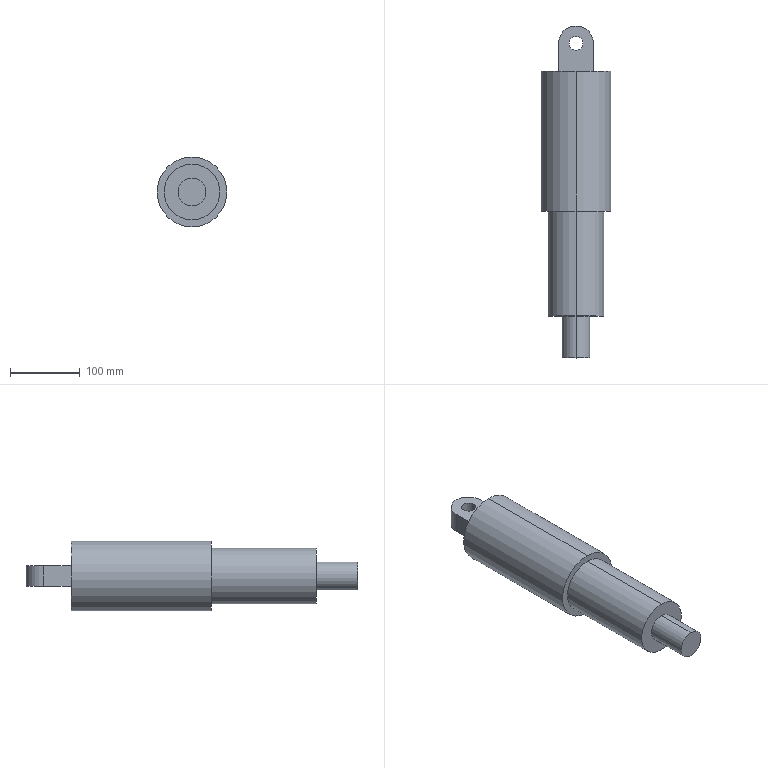Part | SolidWorks | features ICE 1, Revolution 1 | 1 solid | 17 faces | box 100 x 475 x 100 mm | volume 2480204 mm3 | cylinder 9 | plane 8 | commonest cylinder face diameters 20 x2 40 x2 80 x2 100 x2 50 x1
STEP:
#1=CARTESIAN_POINT('',(-10.,450.,15.));
#2=VERTEX_POINT('',#1);
#3=CARTESIAN_POINT('',(10.,450.,15.));
#4=VERTEX_POINT('',#3);
#5=CARTESIAN_POINT('',(0.,450.,15.));
#6=DIRECTION('',(0.,0.,1.));
#7=DIRECTION('',(1.,0.,0.));
#8=AXIS2_PLACEMENT_3D('',#5,#6,#7);
#9=CIRCLE('',#8,10.);
#10=EDGE_CURVE('',#2,#4,#9,.T.);
#11=ORIENTED_EDGE('',*,*,#10,.T.);
#12=CARTESIAN_POINT('',(10.,450.,-15.));
#13=VERTEX_POINT('',#12);
#14=CARTESIAN_POINT('',(10.,450.,15.));
#15=DIRECTION('',(0.,0.,-1.));
#16=VECTOR('',#15,1000.);
#17=LINE('',#14,#16);
#18=EDGE_CURVE('',#4,#13,#17,.T.);
#19=ORIENTED_EDGE('',*,*,#18,.T.);
#20=CARTESIAN_POINT('',(-10.,450.,-15.));
#21=VERTEX_POINT('',#20);
#22=CARTESIAN_POINT('',(0.,450.,-15.));
#23=DIRECTION('',(0.,0.,1.));
#24=DIRECTION('',(1.,0.,0.));
#25=AXIS2_PLACEMENT_3D('',#22,#23,#24);
#26=CIRCLE('',#25,10.);
#27=EDGE_CURVE('',#21,#13,#26,.T.);
#28=ORIENTED_EDGE('',*,*,#27,.F.);
#29=CARTESIAN_POINT('',(-10.,450.,15.));
#30=DIRECTION('',(0.,0.,-1.));
#31=VECTOR('',#30,1000.);
#32=LINE('',#29,#31);
#33=EDGE_CURVE('',#2,#21,#32,.T.);
#34=ORIENTED_EDGE('',*,*,#33,.F.);
#35=EDGE_LOOP('',(#11,#19,#28,#34));
#36=FACE_OUTER_BOUND('',#35,.T.);
#37=CARTESIAN_POINT('',(0.,450.,15.));
#38=DIRECTION('',(0.,0.,-1.));
#39=DIRECTION('',(-1.,0.,0.));
#40=AXIS2_PLACEMENT_3D('',#37,#38,#39);
#41=CYLINDRICAL_SURFACE('',#40,10.);
#42=ADVANCED_FACE('',(#36),#41,.F.);
#43=CARTESIAN_POINT('',(0.,60.,-20.));
#44=VERTEX_POINT('',#43);
#45=CARTESIAN_POINT('',(0.,60.,20.));
#46=VERTEX_POINT('',#45);
#47=CARTESIAN_POINT('',(0.,60.,0.));
#48=DIRECTION('',(0.,-1.,0.));
#49=DIRECTION('',(0.,0.,-1.));
#50=AXIS2_PLACEMENT_3D('',#47,#48,#49);
#51=CIRCLE('',#50,20.);
#52=EDGE_CURVE('',#44,#46,#51,.T.);
#53=ORIENTED_EDGE('',*,*,#52,.T.);
#54=CARTESIAN_POINT('',(0.,0.,20.));
#55=VERTEX_POINT('',#54);
#56=CARTESIAN_POINT('',(0.,0.,20.));
#57=DIRECTION('',(0.,-1.,0.));
#58=VECTOR('',#57,1000.);
#59=LINE('',#56,#58);
#60=EDGE_CURVE('',#46,#55,#59,.T.);
#61=ORIENTED_EDGE('',*,*,#60,.T.);
#62=CARTESIAN_POINT('',(0.,0.,-20.));
#63=VERTEX_POINT('',#62);
#64=CARTESIAN_POINT('',(0.,0.,0.));
#65=DIRECTION('',(0.,-1.,0.));
#66=DIRECTION('',(0.,0.,-1.));
#67=AXIS2_PLACEMENT_3D('',#64,#65,#66);
#68=CIRCLE('',#67,20.);
#69=EDGE_CURVE('',#63,#55,#68,.T.);
#70=ORIENTED_EDGE('',*,*,#69,.F.);
#71=CARTESIAN_POINT('',(0.,0.,-20.));
#72=DIRECTION('',(0.,-1.,0.));
#73=VECTOR('',#72,1000.);
#74=LINE('',#71,#73);
#75=EDGE_CURVE('',#44,#63,#74,.T.);
#76=ORIENTED_EDGE('',*,*,#75,.F.);
#77=EDGE_LOOP('',(#53,#61,#70,#76));
#78=FACE_OUTER_BOUND('',#77,.T.);
#79=CARTESIAN_POINT('',(0.,0.,0.));
#80=DIRECTION('',(0.,-1.,0.));
#81=DIRECTION('',(0.,0.,-1.));
#82=AXIS2_PLACEMENT_3D('',#79,#80,#81);
#83=CYLINDRICAL_SURFACE('',#82,20.);
#84=ADVANCED_FACE('',(#78),#83,.T.);
#85=CARTESIAN_POINT('',(0.,210.,-40.));
#86=VERTEX_POINT('',#85);
#87=CARTESIAN_POINT('',(0.,210.,40.));
#88=VERTEX_POINT('',#87);
#89=CARTESIAN_POINT('',(0.,210.,0.));
#90=DIRECTION('',(0.,-1.,0.));
#91=DIRECTION('',(0.,0.,-1.));
#92=AXIS2_PLACEMENT_3D('',#89,#90,#91);
#93=CIRCLE('',#92,40.);
#94=EDGE_CURVE('',#86,#88,#93,.T.);
#95=ORIENTED_EDGE('',*,*,#94,.T.);
#96=CARTESIAN_POINT('',(0.,60.,40.));
#97=VERTEX_POINT('',#96);
#98=CARTESIAN_POINT('',(0.,0.,40.));
#99=DIRECTION('',(0.,-1.,0.));
#100=VECTOR('',#99,1000.);
#101=LINE('',#98,#100);
#102=EDGE_CURVE('',#88,#97,#101,.T.);
#103=ORIENTED_EDGE('',*,*,#102,.T.);
#104=CARTESIAN_POINT('',(0.,60.,-40.));
#105=VERTEX_POINT('',#104);
#106=CARTESIAN_POINT('',(0.,60.,0.));
#107=DIRECTION('',(0.,-1.,0.));
#108=DIRECTION('',(0.,0.,-1.));
#109=AXIS2_PLACEMENT_3D('',#106,#107,#108);
#110=CIRCLE('',#109,40.);
#111=EDGE_CURVE('',#105,#97,#110,.T.);
#112=ORIENTED_EDGE('',*,*,#111,.F.);
#113=CARTESIAN_POINT('',(0.,0.,-40.));
#114=DIRECTION('',(0.,-1.,0.));
#115=VECTOR('',#114,1000.);
#116=LINE('',#113,#115);
#117=EDGE_CURVE('',#86,#105,#116,.T.);
#118=ORIENTED_EDGE('',*,*,#117,.F.);
#119=EDGE_LOOP('',(#95,#103,#112,#118));
#120=FACE_OUTER_BOUND('',#119,.T.);
#121=CARTESIAN_POINT('',(0.,0.,0.));
#122=DIRECTION('',(0.,-1.,0.));
#123=DIRECTION('',(0.,0.,-1.));
#124=AXIS2_PLACEMENT_3D('',#121,#122,#123);
#125=CYLINDRICAL_SURFACE('',#124,40.);
#126=ADVANCED_FACE('',(#120),#125,.T.);
#127=CARTESIAN_POINT('',(0.,410.,-50.));
#128=VERTEX_POINT('',#127);
#129=CARTESIAN_POINT('',(0.,410.,50.));
#130=VERTEX_POINT('',#129);
#131=CARTESIAN_POINT('',(0.,410.,0.));
#132=DIRECTION('',(0.,-1.,0.));
#133=DIRECTION('',(0.,0.,-1.));
#134=AXIS2_PLACEMENT_3D('',#131,#132,#133);
#135=CIRCLE('',#134,50.);
#136=EDGE_CURVE('',#128,#130,#135,.T.);
#137=ORIENTED_EDGE('',*,*,#136,.T.);
#138=CARTESIAN_POINT('',(0.,210.,50.));
#139=VERTEX_POINT('',#138);
#140=CARTESIAN_POINT('',(0.,0.,50.));
#141=DIRECTION('',(0.,-1.,0.));
#142=VECTOR('',#141,1000.);
#143=LINE('',#140,#142);
#144=EDGE_CURVE('',#130,#139,#143,.T.);
#145=ORIENTED_EDGE('',*,*,#144,.T.);
#146=CARTESIAN_POINT('',(0.,210.,-50.));
#147=VERTEX_POINT('',#146);
#148=CARTESIAN_POINT('',(0.,210.,0.));
#149=DIRECTION('',(0.,-1.,0.));
#150=DIRECTION('',(0.,0.,-1.));
#151=AXIS2_PLACEMENT_3D('',#148,#149,#150);
#152=CIRCLE('',#151,50.);
#153=EDGE_CURVE('',#147,#139,#152,.T.);
#154=ORIENTED_EDGE('',*,*,#153,.F.);
#155=CARTESIAN_POINT('',(0.,0.,-50.));
#156=DIRECTION('',(0.,-1.,0.));
#157=VECTOR('',#156,1000.);
#158=LINE('',#155,#157);
#159=EDGE_CURVE('',#128,#147,#158,.T.);
#160=ORIENTED_EDGE('',*,*,#159,.F.);
#161=EDGE_LOOP('',(#137,#145,#154,#160));
#162=FACE_OUTER_BOUND('',#161,.T.);
#163=CARTESIAN_POINT('',(0.,0.,0.));
#164=DIRECTION('',(0.,-1.,0.));
#165=DIRECTION('',(0.,0.,-1.));
#166=AXIS2_PLACEMENT_3D('',#163,#164,#165);
#167=CYLINDRICAL_SURFACE('',#166,50.);
#168=ADVANCED_FACE('',(#162),#167,.T.);
#169=ORIENTED_EDGE('',*,*,#136,.F.);
#170=CARTESIAN_POINT('',(0.,410.,0.));
#171=DIRECTION('',(0.,-1.,0.));
#172=DIRECTION('',(0.,0.,-1.));
#173=AXIS2_PLACEMENT_3D('',#170,#171,#172);
#174=CIRCLE('',#173,50.);
#175=EDGE_CURVE('',#130,#128,#174,.T.);
#176=ORIENTED_EDGE('',*,*,#175,.F.);
#177=EDGE_LOOP('',(#169,#176));
#178=FACE_OUTER_BOUND('',#177,.T.);
#179=CARTESIAN_POINT('',(-25.,410.,15.));
#180=VERTEX_POINT('',#179);
#181=CARTESIAN_POINT('',(-25.,410.,-15.));
#182=VERTEX_POINT('',#181);
#183=CARTESIAN_POINT('',(-25.,410.,15.));
#184=DIRECTION('',(0.,0.,-1.));
#185=VECTOR('',#184,1000.);
#186=LINE('',#183,#185);
#187=EDGE_CURVE('',#180,#182,#186,.T.);
#188=ORIENTED_EDGE('',*,*,#187,.T.);
#189=CARTESIAN_POINT('',(25.,410.,-15.));
#190=VERTEX_POINT('',#189);
#191=CARTESIAN_POINT('',(-25.,410.,-15.));
#192=DIRECTION('',(1.,0.,0.));
#193=VECTOR('',#192,1000.);
#194=LINE('',#191,#193);
#195=EDGE_CURVE('',#182,#190,#194,.T.);
#196=ORIENTED_EDGE('',*,*,#195,.T.);
#197=CARTESIAN_POINT('',(25.,410.,15.));
#198=VERTEX_POINT('',#197);
#199=CARTESIAN_POINT('',(25.,410.,15.));
#200=DIRECTION('',(0.,0.,-1.));
#201=VECTOR('',#200,1000.);
#202=LINE('',#199,#201);
#203=EDGE_CURVE('',#198,#190,#202,.T.);
#204=ORIENTED_EDGE('',*,*,#203,.F.);
#205=CARTESIAN_POINT('',(-25.,410.,15.));
#206=DIRECTION('',(1.,0.,0.));
#207=VECTOR('',#206,1000.);
#208=LINE('',#205,#207);
#209=EDGE_CURVE('',#180,#198,#208,.T.);
#210=ORIENTED_EDGE('',*,*,#209,.F.);
#211=EDGE_LOOP('',(#188,#196,#204,#210));
#212=FACE_BOUND('',#211,.T.);
#213=CARTESIAN_POINT('',(0.,410.,0.));
#214=DIRECTION('',(0.,1.,0.));
#215=DIRECTION('',(0.,0.,1.));
#216=AXIS2_PLACEMENT_3D('',#213,#214,#215);
#217=PLANE('',#216);
#218=ADVANCED_FACE('',(#178,#212),#217,.T.);
#219=ORIENTED_EDGE('',*,*,#69,.T.);
#220=CARTESIAN_POINT('',(0.,0.,0.));
#221=DIRECTION('',(0.,-1.,0.));
#222=DIRECTION('',(0.,0.,-1.));
#223=AXIS2_PLACEMENT_3D('',#220,#221,#222);
#224=CIRCLE('',#223,20.);
#225=EDGE_CURVE('',#55,#63,#224,.T.);
#226=ORIENTED_EDGE('',*,*,#225,.T.);
#227=EDGE_LOOP('',(#219,#226));
#228=FACE_OUTER_BOUND('',#227,.T.);
#229=CARTESIAN_POINT('',(20.,0.,0.));
#230=DIRECTION('',(0.,-1.,0.));
#231=DIRECTION('',(0.,0.,-1.));
#232=AXIS2_PLACEMENT_3D('',#229,#230,#231);
#233=PLANE('',#232);
#234=ADVANCED_FACE('',(#228),#233,.T.);
#235=ORIENTED_EDGE('',*,*,#144,.F.);
#236=ORIENTED_EDGE('',*,*,#175,.T.);
#237=ORIENTED_EDGE('',*,*,#159,.T.);
#238=CARTESIAN_POINT('',(0.,210.,0.));
#239=DIRECTION('',(0.,-1.,0.));
#240=DIRECTION('',(0.,0.,-1.));
#241=AXIS2_PLACEMENT_3D('',#238,#239,#240);
#242=CIRCLE('',#241,50.);
#243=EDGE_CURVE('',#139,#147,#242,.T.);
#244=ORIENTED_EDGE('',*,*,#243,.F.);
#245=EDGE_LOOP('',(#235,#236,#237,#244));
#246=FACE_OUTER_BOUND('',#245,.T.);
#247=CARTESIAN_POINT('',(0.,0.,0.));
#248=DIRECTION('',(0.,-1.,0.));
#249=DIRECTION('',(0.,0.,-1.));
#250=AXIS2_PLACEMENT_3D('',#247,#248,#249);
#251=CYLINDRICAL_SURFACE('',#250,50.);
#252=ADVANCED_FACE('',(#246),#251,.T.);
#253=ORIENTED_EDGE('',*,*,#153,.T.);
#254=ORIENTED_EDGE('',*,*,#243,.T.);
#255=EDGE_LOOP('',(#253,#254));
#256=FACE_OUTER_BOUND('',#255,.T.);
#257=ORIENTED_EDGE('',*,*,#94,.F.);
#258=CARTESIAN_POINT('',(0.,210.,0.));
#259=DIRECTION('',(0.,-1.,0.));
#260=DIRECTION('',(0.,0.,-1.));
#261=AXIS2_PLACEMENT_3D('',#258,#259,#260);
#262=CIRCLE('',#261,40.);
#263=EDGE_CURVE('',#88,#86,#262,.T.);
#264=ORIENTED_EDGE('',*,*,#263,.F.);
#265=EDGE_LOOP('',(#257,#264));
#266=FACE_BOUND('',#265,.T.);
#267=CARTESIAN_POINT('',(50.,210.,0.));
#268=DIRECTION('',(0.,-1.,0.));
#269=DIRECTION('',(0.,0.,-1.));
#270=AXIS2_PLACEMENT_3D('',#267,#268,#269);
#271=PLANE('',#270);
#272=ADVANCED_FACE('',(#256,#266),#271,.T.);
#273=ORIENTED_EDGE('',*,*,#102,.F.);
#274=ORIENTED_EDGE('',*,*,#263,.T.);
#275=ORIENTED_EDGE('',*,*,#117,.T.);
#276=CARTESIAN_POINT('',(0.,60.,0.));
#277=DIRECTION('',(0.,-1.,0.));
#278=DIRECTION('',(0.,0.,-1.));
#279=AXIS2_PLACEMENT_3D('',#276,#277,#278);
#280=CIRCLE('',#279,40.);
#281=EDGE_CURVE('',#97,#105,#280,.T.);
#282=ORIENTED_EDGE('',*,*,#281,.F.);
#283=EDGE_LOOP('',(#273,#274,#275,#282));
#284=FACE_OUTER_BOUND('',#283,.T.);
#285=CARTESIAN_POINT('',(0.,0.,0.));
#286=DIRECTION('',(0.,-1.,0.));
#287=DIRECTION('',(0.,0.,-1.));
#288=AXIS2_PLACEMENT_3D('',#285,#286,#287);
#289=CYLINDRICAL_SURFACE('',#288,40.);
#290=ADVANCED_FACE('',(#284),#289,.T.);
#291=ORIENTED_EDGE('',*,*,#111,.T.);
#292=ORIENTED_EDGE('',*,*,#281,.T.);
#293=EDGE_LOOP('',(#291,#292));
#294=FACE_OUTER_BOUND('',#293,.T.);
#295=ORIENTED_EDGE('',*,*,#52,.F.);
#296=CARTESIAN_POINT('',(0.,60.,0.));
#297=DIRECTION('',(0.,-1.,0.));
#298=DIRECTION('',(0.,0.,-1.));
#299=AXIS2_PLACEMENT_3D('',#296,#297,#298);
#300=CIRCLE('',#299,20.);
#301=EDGE_CURVE('',#46,#44,#300,.T.);
#302=ORIENTED_EDGE('',*,*,#301,.F.);
#303=EDGE_LOOP('',(#295,#302));
#304=FACE_BOUND('',#303,.T.);
#305=CARTESIAN_POINT('',(40.,60.,0.));
#306=DIRECTION('',(0.,-1.,0.));
#307=DIRECTION('',(0.,0.,-1.));
#308=AXIS2_PLACEMENT_3D('',#305,#306,#307);
#309=PLANE('',#308);
#310=ADVANCED_FACE('',(#294,#304),#309,.T.);
#311=ORIENTED_EDGE('',*,*,#60,.F.);
#312=ORIENTED_EDGE('',*,*,#301,.T.);
#313=ORIENTED_EDGE('',*,*,#75,.T.);
#314=ORIENTED_EDGE('',*,*,#225,.F.);
#315=EDGE_LOOP('',(#311,#312,#313,#314));
#316=FACE_OUTER_BOUND('',#315,.T.);
#317=CARTESIAN_POINT('',(0.,0.,0.));
#318=DIRECTION('',(0.,-1.,0.));
#319=DIRECTION('',(0.,0.,-1.));
#320=AXIS2_PLACEMENT_3D('',#317,#318,#319);
#321=CYLINDRICAL_SURFACE('',#320,20.);
#322=ADVANCED_FACE('',(#316),#321,.T.);
#323=CARTESIAN_POINT('',(25.,450.,15.));
#324=VERTEX_POINT('',#323);
#325=CARTESIAN_POINT('',(-25.,450.,15.));
#326=VERTEX_POINT('',#325);
#327=CARTESIAN_POINT('',(0.,450.,15.));
#328=DIRECTION('',(0.,0.,1.));
#329=DIRECTION('',(1.,0.,0.));
#330=AXIS2_PLACEMENT_3D('',#327,#328,#329);
#331=CIRCLE('',#330,25.);
#332=EDGE_CURVE('',#324,#326,#331,.T.);
#333=ORIENTED_EDGE('',*,*,#332,.T.);
#334=CARTESIAN_POINT('',(-25.,450.,15.));
#335=DIRECTION('',(0.,-1.,0.));
#336=VECTOR('',#335,1000.);
#337=LINE('',#334,#336);
#338=EDGE_CURVE('',#326,#180,#337,.T.);
#339=ORIENTED_EDGE('',*,*,#338,.T.);
#340=ORIENTED_EDGE('',*,*,#209,.T.);
#341=CARTESIAN_POINT('',(25.,410.,15.));
#342=DIRECTION('',(0.,1.,0.));
#343=VECTOR('',#342,1000.);
#344=LINE('',#341,#343);
#345=EDGE_CURVE('',#198,#324,#344,.T.);
#346=ORIENTED_EDGE('',*,*,#345,.T.);
#347=EDGE_LOOP('',(#333,#339,#340,#346));
#348=FACE_OUTER_BOUND('',#347,.T.);
#349=ORIENTED_EDGE('',*,*,#10,.F.);
#350=CARTESIAN_POINT('',(0.,450.,15.));
#351=DIRECTION('',(0.,0.,1.));
#352=DIRECTION('',(1.,0.,0.));
#353=AXIS2_PLACEMENT_3D('',#350,#351,#352);
#354=CIRCLE('',#353,10.);
#355=EDGE_CURVE('',#4,#2,#354,.T.);
#356=ORIENTED_EDGE('',*,*,#355,.F.);
#357=EDGE_LOOP('',(#349,#356));
#358=FACE_BOUND('',#357,.T.);
#359=CARTESIAN_POINT('',(0.,450.,15.));
#360=DIRECTION('',(0.,0.,1.));
#361=DIRECTION('',(1.,0.,0.));
#362=AXIS2_PLACEMENT_3D('',#359,#360,#361);
#363=PLANE('',#362);
#364=ADVANCED_FACE('',(#348,#358),#363,.T.);
#365=CARTESIAN_POINT('',(25.,450.,-15.));
#366=VERTEX_POINT('',#365);
#367=CARTESIAN_POINT('',(-25.,450.,-15.));
#368=VERTEX_POINT('',#367);
#369=CARTESIAN_POINT('',(0.,450.,-15.));
#370=DIRECTION('',(0.,0.,1.));
#371=DIRECTION('',(1.,0.,0.));
#372=AXIS2_PLACEMENT_3D('',#369,#370,#371);
#373=CIRCLE('',#372,25.);
#374=EDGE_CURVE('',#366,#368,#373,.T.);
#375=ORIENTED_EDGE('',*,*,#374,.F.);
#376=CARTESIAN_POINT('',(25.,410.,-15.));
#377=DIRECTION('',(0.,1.,0.));
#378=VECTOR('',#377,1000.);
#379=LINE('',#376,#378);
#380=EDGE_CURVE('',#190,#366,#379,.T.);
#381=ORIENTED_EDGE('',*,*,#380,.F.);
#382=ORIENTED_EDGE('',*,*,#195,.F.);
#383=CARTESIAN_POINT('',(-25.,450.,-15.));
#384=DIRECTION('',(0.,-1.,0.));
#385=VECTOR('',#384,1000.);
#386=LINE('',#383,#385);
#387=EDGE_CURVE('',#368,#182,#386,.T.);
#388=ORIENTED_EDGE('',*,*,#387,.F.);
#389=EDGE_LOOP('',(#375,#381,#382,#388));
#390=FACE_OUTER_BOUND('',#389,.T.);
#391=ORIENTED_EDGE('',*,*,#27,.T.);
#392=CARTESIAN_POINT('',(0.,450.,-15.));
#393=DIRECTION('',(0.,0.,1.));
#394=DIRECTION('',(1.,0.,0.));
#395=AXIS2_PLACEMENT_3D('',#392,#393,#394);
#396=CIRCLE('',#395,10.);
#397=EDGE_CURVE('',#13,#21,#396,.T.);
#398=ORIENTED_EDGE('',*,*,#397,.T.);
#399=EDGE_LOOP('',(#391,#398));
#400=FACE_BOUND('',#399,.T.);
#401=CARTESIAN_POINT('',(0.,450.,-15.));
#402=DIRECTION('',(0.,0.,1.));
#403=DIRECTION('',(1.,0.,0.));
#404=AXIS2_PLACEMENT_3D('',#401,#402,#403);
#405=PLANE('',#404);
#406=ADVANCED_FACE('',(#390,#400),#405,.F.);
#407=ORIENTED_EDGE('',*,*,#374,.T.);
#408=CARTESIAN_POINT('',(-25.,450.,15.));
#409=DIRECTION('',(0.,0.,-1.));
#410=VECTOR('',#409,1000.);
#411=LINE('',#408,#410);
#412=EDGE_CURVE('',#326,#368,#411,.T.);
#413=ORIENTED_EDGE('',*,*,#412,.F.);
#414=ORIENTED_EDGE('',*,*,#332,.F.);
#415=CARTESIAN_POINT('',(25.,450.,15.));
#416=DIRECTION('',(0.,0.,-1.));
#417=VECTOR('',#416,1000.);
#418=LINE('',#415,#417);
#419=EDGE_CURVE('',#324,#366,#418,.T.);
#420=ORIENTED_EDGE('',*,*,#419,.T.);
#421=EDGE_LOOP('',(#407,#413,#414,#420));
#422=FACE_OUTER_BOUND('',#421,.T.);
#423=CARTESIAN_POINT('',(0.,450.,15.));
#424=DIRECTION('',(0.,0.,-1.));
#425=DIRECTION('',(-1.,0.,0.));
#426=AXIS2_PLACEMENT_3D('',#423,#424,#425);
#427=CYLINDRICAL_SURFACE('',#426,25.);
#428=ADVANCED_FACE('',(#422),#427,.T.);
#429=ORIENTED_EDGE('',*,*,#387,.T.);
#430=ORIENTED_EDGE('',*,*,#187,.F.);
#431=ORIENTED_EDGE('',*,*,#338,.F.);
#432=ORIENTED_EDGE('',*,*,#412,.T.);
#433=EDGE_LOOP('',(#429,#430,#431,#432));
#434=FACE_OUTER_BOUND('',#433,.T.);
#435=CARTESIAN_POINT('',(-25.,450.,15.));
#436=DIRECTION('',(1.,0.,0.));
#437=DIRECTION('',(0.,1.,0.));
#438=AXIS2_PLACEMENT_3D('',#435,#436,#437);
#439=PLANE('',#438);
#440=ADVANCED_FACE('',(#434),#439,.F.);
#441=ORIENTED_EDGE('',*,*,#380,.T.);
#442=ORIENTED_EDGE('',*,*,#419,.F.);
#443=ORIENTED_EDGE('',*,*,#345,.F.);
#444=ORIENTED_EDGE('',*,*,#203,.T.);
#445=EDGE_LOOP('',(#441,#442,#443,#444));
#446=FACE_OUTER_BOUND('',#445,.T.);
#447=CARTESIAN_POINT('',(25.,410.,15.));
#448=DIRECTION('',(-1.,0.,0.));
#449=DIRECTION('',(0.,0.,1.));
#450=AXIS2_PLACEMENT_3D('',#447,#448,#449);
#451=PLANE('',#450);
#452=ADVANCED_FACE('',(#446),#451,.F.);
#453=ORIENTED_EDGE('',*,*,#18,.F.);
#454=ORIENTED_EDGE('',*,*,#355,.T.);
#455=ORIENTED_EDGE('',*,*,#33,.T.);
#456=ORIENTED_EDGE('',*,*,#397,.F.);
#457=EDGE_LOOP('',(#453,#454,#455,#456));
#458=FACE_OUTER_BOUND('',#457,.T.);
#459=CARTESIAN_POINT('',(0.,450.,15.));
#460=DIRECTION('',(0.,0.,-1.));
#461=DIRECTION('',(-1.,0.,0.));
#462=AXIS2_PLACEMENT_3D('',#459,#460,#461);
#463=CYLINDRICAL_SURFACE('',#462,10.);
#464=ADVANCED_FACE('',(#458),#463,.F.);
#465=CLOSED_SHELL('',(#42,#84,#126,#168,#218,#234,#252,#272,#290,#310,#322,#364,#406,#428,#440,#452,#464));
#466=MANIFOLD_SOLID_BREP('',#465);
#467=CARTESIAN_POINT('',(0.,0.,0.));
#468=DIRECTION('',(0.,0.,1.));
#469=DIRECTION('',(1.,0.,0.));
#470=AXIS2_PLACEMENT_3D('',#467,#468,#469);
#471=(LENGTH_UNIT()NAMED_UNIT(*)SI_UNIT(.MILLI.,.METRE.));
#472=UNCERTAINTY_MEASURE_WITH_UNIT(LENGTH_MEASURE(0.00001),#471,'','');
#473=(NAMED_UNIT(*)PLANE_ANGLE_UNIT()SI_UNIT($,.RADIAN.));
#474=(NAMED_UNIT(*)SI_UNIT($,.STERADIAN.)SOLID_ANGLE_UNIT());
#475=(GEOMETRIC_REPRESENTATION_CONTEXT(3)GLOBAL_UNCERTAINTY_ASSIGNED_CONTEXT((#472))GLOBAL_UNIT_ASSIGNED_CONTEXT((#471,#473,#474))REPRESENTATION_CONTEXT('',''));
#476=ADVANCED_BREP_SHAPE_REPRESENTATION('',(#466,#470),#475);